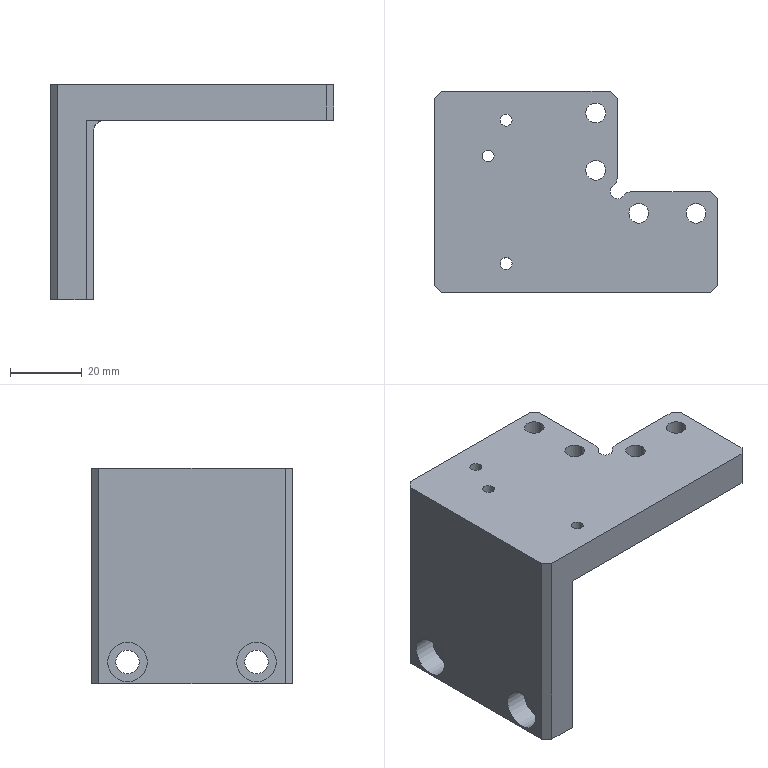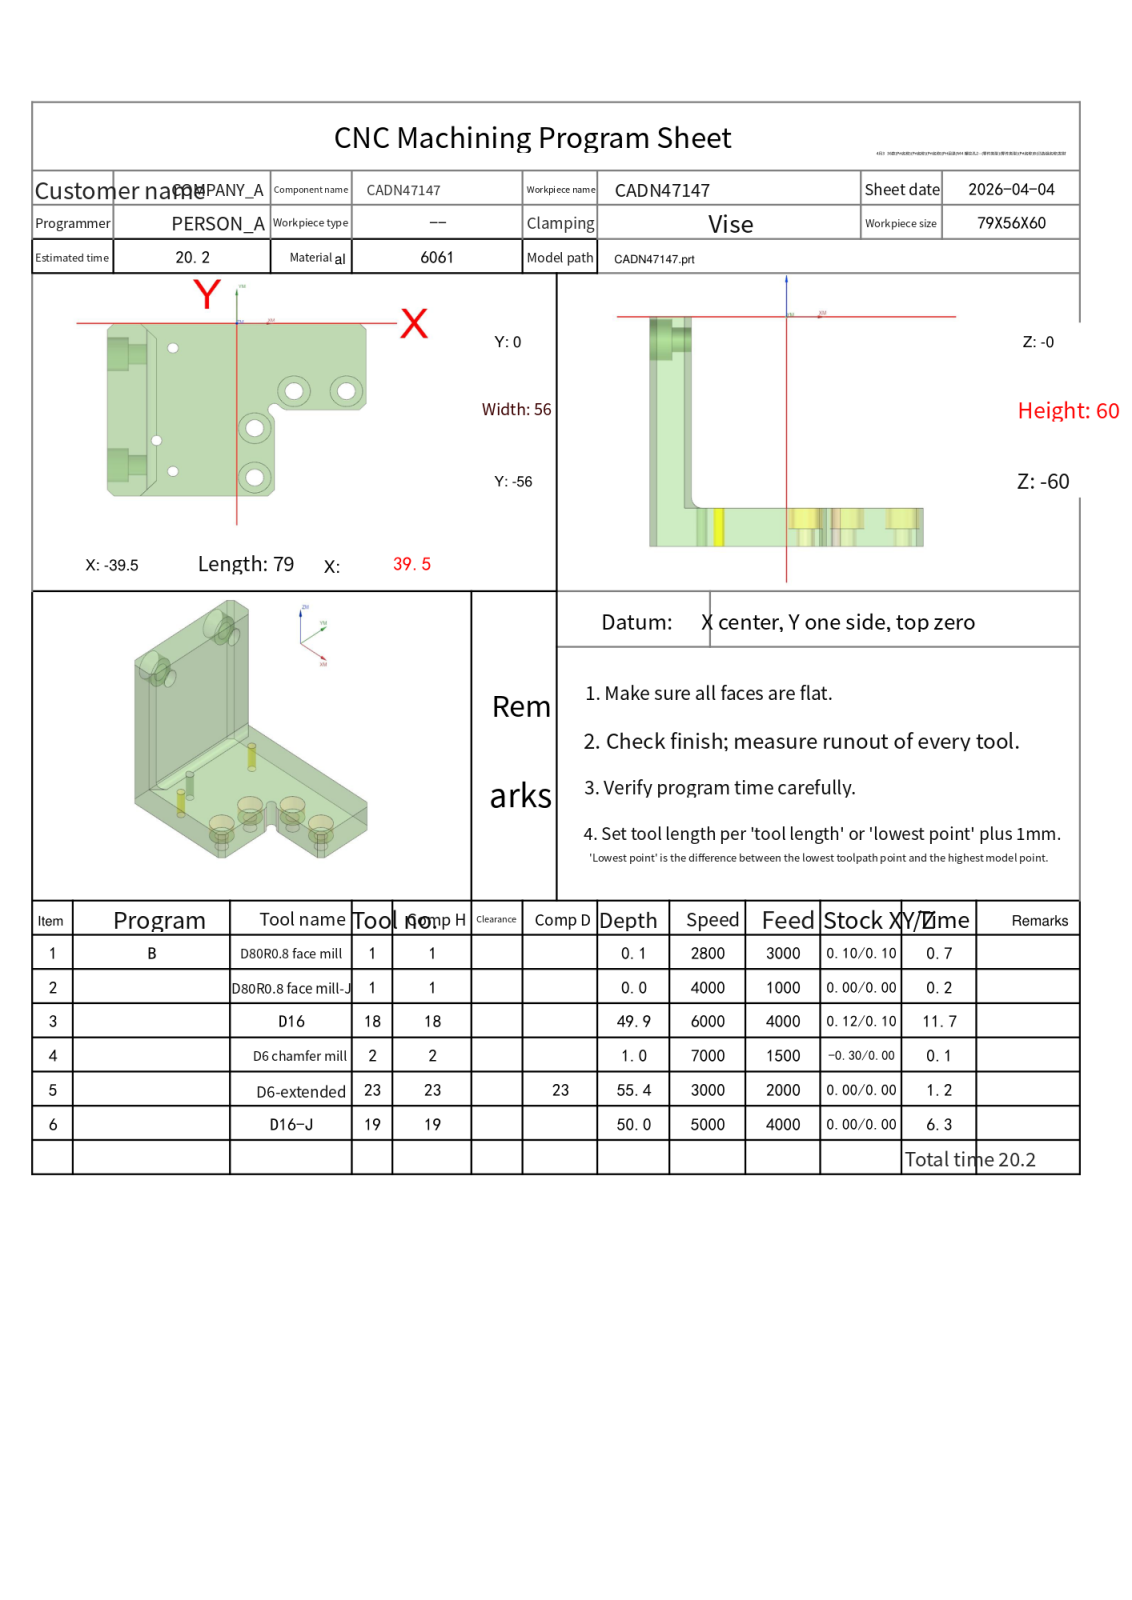NC program | NX | posted by the shop | part box 79 x 56 x 60 mm
Lines 11359 to 12639 of 15895:
N6 T19 M06
(D16-J  D=16. R=0. H=19 ce=0.40 di=0.00)
G00 G90 G54 X-.77 Y11.2 M03 S5000
G43 H19 Z14.5
M08
Z-48.5
G01 Z-50. F1000.
Y4.8
G03 X2.43 Y1.6 I3.2 J0.0
G01 X37.503
G02 X38.629 Y1.134 I-.003 J-1.6
G01 X40.634 Y-.871
G02 X41.1 Y-1.997 I-1.134 J-1.129
G01 Y-26.003
G02 X40.634 Y-27.129 I-1.6 J.003
G01 X38.629 Y-29.134
G02 X37.503 Y-29.6 I-1.129 J1.134
G01 X13.1
Y-54.003
G02 X12.634 Y-55.129 I-1.6 J.003
G01 X10.629 Y-57.134
G02 X9.503 Y-57.6 I-1.129 J1.134
G01 X-18.45
G02 X-18.768 Y-57.28 I.001 J.32
X-18.675 Y-57.055 I.32 J0.0
G01 X-16.1 Y-54.479
Y-1.521
X-18.675 Y1.055
G02 X-18.768 Y1.28 I.227 J.225
X-18.45 Y1.6 I.32 J0.0
G01 X5.768
G02 X6.898 Y1.132 I-.001 J-1.6
G01 X13.962 Y-5.932
G03 X15.092 Y-6.4 I1.131 J1.132
G01 X31.504
G02 X33.1 Y-7.996 I-.004 J-1.6
G01 Y-20.004
G02 X31.504 Y-21.6 I-1.6 J.004
G01 X13.1
G03 X5.1 Y-29.6 I0.0 J-8.
G01 Y-48.004
G02 X3.504 Y-49.6 I-1.6 J.004
G01 X-6.504
G02 X-8.1 Y-48.004 I.004 J1.6
G01 Y-7.996
G02 X-6.504 Y-6.4 I1.6 J-.004
G01 X4.94
G02 X6.06 Y-7.52 I0.0 J-1.12
X6.016 Y-7.831 I-1.12 J0.0
G01 X4.266 Y-13.878
G03 X4.203 Y-14.322 I1.537 J-.444
X4.367 Y-15.027 I1.6 J0.0
G02 X4.481 Y-15.52 I-1.005 J-.493
X4.001 Y-16.439 I-1.12 J0.0
G03 X2.552 Y-17.569 I9.099 J-13.161
G02 X1.5 Y-17.964 I-1.052 J1.206
X-.1 Y-16.367 I0.0 J1.6
G01 Y-15.996
G02 X1.496 Y-14.4 I1.6 J-.004
G01 X3.364
G02 X4.047 Y-14.635 I-.003 J-1.12
X4.481 Y-15.499 I-.686 J-.885
G03 X7.68 Y-18.64 I3.199 J.059
G01 X7.74 Y-18.639
Z-48.5
G00 Z14.5
G00 G90 X-23.903 Y9.001 M03 S5000
Z9.5
Z-8.4
G01 Z-9.4 F1000.
G41 D19
X-24.028 Y8.844
G03 X-24.546 Y7.354 I1.882 J-1.49
X-23.843 Y5.657 I2.4 J0.0
G01 X-21.843 Y3.657
G02 X-19.5 Y-2. I-5.657 J-5.657
G01 Y-54.
G02 X-21.847 Y-59.661 I-8. J0.0
G01 X-23.843 Y-61.657
G03 X-24.546 Y-63.354 I1.697 J-1.697
X-24.028 Y-64.844 I2.4 J0.0
G01 G40 X-23.903 Y-65.001
Z-8.4
G00 Z9.5
Y9.001
Z-17.8
G01 Z-18.8
G41 D19
X-24.028 Y8.844
G03 X-24.546 Y7.354 I1.882 J-1.49
X-23.843 Y5.657 I2.4 J0.0
G01 X-21.843 Y3.657
G02 X-19.5 Y-2. I-5.657 J-5.657
G01 Y-54.
G02 X-21.847 Y-59.661 I-8. J0.0
G01 X-23.843 Y-61.657
G03 X-24.546 Y-63.354 I1.697 J-1.697
X-24.028 Y-64.844 I2.4 J0.0
G01 G40 X-23.903 Y-65.001
Z-17.8
G00 Z9.5
Y9.001
Z-27.2
G01 Z-28.2
G41 D19
X-24.028 Y8.844
G03 X-24.546 Y7.354 I1.882 J-1.49
X-23.843 Y5.657 I2.4 J0.0
G01 X-21.843 Y3.657
G02 X-19.5 Y-2. I-5.657 J-5.657
G01 Y-54.
G02 X-21.847 Y-59.661 I-8. J0.0
G01 X-23.843 Y-61.657
G03 X-24.546 Y-63.354 I1.697 J-1.697
X-24.028 Y-64.844 I2.4 J0.0
G01 G40 X-23.903 Y-65.001
Z-27.2
G00 Z9.5
Y9.001
Z-36.6
G01 Z-37.6
G41 D19
X-24.028 Y8.844
G03 X-24.546 Y7.354 I1.882 J-1.49
X-23.843 Y5.657 I2.4 J0.0
G01 X-21.843 Y3.657
G02 X-19.5 Y-2. I-5.657 J-5.657
G01 Y-54.
G02 X-21.847 Y-59.661 I-8. J0.0
G01 X-23.843 Y-61.657
G03 X-24.546 Y-63.354 I1.697 J-1.697
X-24.028 Y-64.844 I2.4 J0.0
G01 G40 X-23.903 Y-65.001
Z-36.6
G00 Z9.5
Y9.001
Z-46.
G01 Z-47.
G41 D19
X-24.028 Y8.844
G03 X-24.546 Y7.354 I1.882 J-1.49
X-23.843 Y5.657 I2.4 J0.0
G01 X-21.843 Y3.657
G02 X-19.5 Y-2. I-5.657 J-5.657
G01 Y-54.
G02 X-21.847 Y-59.661 I-8. J0.0
G01 X-23.843 Y-61.657
G03 X-24.546 Y-63.354 I1.697 J-1.697
X-24.028 Y-64.844 I2.4 J0.0
G01 G40 X-23.903 Y-65.001
Z-46.
G00 Z9.5
G00 G90 X-26.925 Y11.391 M03 S5000
Z14.5
Z-49.
G01 Z-50. F1000.
G41 D19
X-26.983 Y11.2
G03 X-27.124 Y10.263 I3.06 J-.937
X-26.186 Y8. I3.2 J0.0
G01 X-16.5 Y-1.686
Y-54.314
X-26.186 Y-64.
G03 X-27.124 Y-66.263 I2.263 J-2.263
X-26.983 Y-67.2 I3.2 J0.0
G01 G40 X-26.925 Y-67.391
Z-49.
G00 Z14.5
G00 G90 X-34.428 Y16.241 M03 S5000
Z14.5
Z-46.515
G01 Z-47.015 F4000.
X-24.723 Y6.55
X-23.895 Y5.724
X-23.836 Y5.664
X-21.836 Y3.664
X-21.721 Y3.546
G02 X-19.489 Y-2.001 I-5.778 J-5.547
G01 Y-2.032
X-19.49 Y-2.755
Y-53.245
Y-53.642
Y-53.948
Y-54.006
G02 X-21.755 Y-59.582 I-7.994 J0.0
G01 X-21.836 Y-59.664
X-23.836 Y-61.664
X-24.723 Y-62.55
Z-47.03
X-23.836 Y-61.664
X-21.835 Y-59.663
X-21.755 Y-59.582
G03 X-19.49 Y-54.006 I-5.729 J5.576
G01 Y-53.948
Y-53.642
Y-53.248
Y-2.752
X-19.489 Y-2.032
Y-1.999
G03 X-21.721 Y3.546 I-8.006 J0.0
G01 X-21.835 Y3.663
X-23.836 Y5.664
X-23.895 Y5.724
X-24.723 Y6.55
Z-47.045
X-23.895 Y5.724
X-23.836 Y5.664
X-21.835 Y3.663
X-21.721 Y3.546
G02 X-19.489 Y-1.998 I-5.77 J-5.544
G01 Y-2.032
X-19.49 Y-2.488
Y-53.948
X-19.489 Y-54.005
G02 X-21.755 Y-59.582 I-7.996 J0.0
G01 X-21.835 Y-59.663
X-23.836 Y-61.664
X-24.723 Y-62.55
Z-47.06
X-23.836 Y-61.664
X-21.835 Y-59.663
X-21.755 Y-59.582
G03 X-19.489 Y-54.004 I-5.732 J5.578
G01 Y-53.948
Y-2.488
Y-2.042
X-19.488 Y-2.032
Y-2.
G03 X-21.721 Y3.546 I-8.005 J0.0
G01 X-21.835 Y3.663
X-23.836 Y5.664
X-23.895 Y5.724
X-24.723 Y6.55
Z-47.075
X-23.895 Y5.724
X-23.836 Y5.664
X-21.835 Y3.662
X-21.721 Y3.546
G02 X-19.489 Y-1.993 I-5.759 J-5.54
G01 Y-2.072
Y-53.968
Y-54.004
G02 X-21.755 Y-59.582 I-7.998 J0.0
G01 X-21.835 Y-59.662
X-23.836 Y-61.664
X-24.723 Y-62.55
Z-47.09
X-23.836 Y-61.664
X-21.834 Y-59.662
X-21.755 Y-59.582
G03 X-19.489 Y-54.004 I-5.731 J5.578
G01 Y-53.968
Y-2.042
Y-2.006
G03 X-21.721 Y3.546 I-8.023 J0.0
G01 X-21.834 Y3.662
X-23.836 Y5.664
X-23.895 Y5.724
X-24.723 Y6.55
Z-47.105
X-23.895 Y5.724
X-23.836 Y5.664
X-21.834 Y3.662
X-21.721 Y3.546
G02 X-19.488 Y-1.98 I-5.722 J-5.526
G01 Y-2.042
Y-53.968
Y-54.004
G02 X-21.755 Y-59.582 I-7.996 J0.0
G01 X-21.834 Y-59.662
X-23.836 Y-61.664
X-23.895 Y-61.724
X-24.723 Y-62.55
Z-47.12
X-23.895 Y-61.724
X-23.836 Y-61.664
X-21.834 Y-59.661
X-21.755 Y-59.582
G03 X-19.488 Y-54.005 I-5.724 J5.577
G01 Y-53.968
Y-2.042
X-19.487 Y-1.98
G03 X-21.721 Y3.546 I-7.955 J0.0
G01 X-21.834 Y3.661
X-23.836 Y5.664
X-23.895 Y5.724
X-24.723 Y6.55
Z-47.135
X-23.895 Y5.724
X-23.836 Y5.664
X-21.833 Y3.661
X-21.721 Y3.546
G02 X-19.482 Y-2.009 I-5.772 J-5.555
G01 Y-2.031
X-19.487 Y-2.042
Y-53.968
Y-54.006
G02 X-21.755 Y-59.582 I-7.987 J0.0
G01 X-21.833 Y-59.661
X-23.836 Y-61.664
X-23.895 Y-61.724
X-24.723 Y-62.55
Z-47.15
X-23.895 Y-61.724
X-23.836 Y-61.664
X-21.832 Y-59.66
X-21.755 Y-59.582
G03 X-19.486 Y-54.006 I-5.716 J5.575
G01 Y-53.968
Y-2.042
X-19.481 Y-2.031
Y-2.009
G03 X-21.721 Y3.546 I-8.009 J0.0
G01 X-21.832 Y3.66
X-23.836 Y5.664
X-23.895 Y5.724
X-24.723 Y6.55
Z-47.165
X-23.895 Y5.724
X-23.836 Y5.664
X-21.831 Y3.659
X-21.721 Y3.546
G02 X-19.485 Y-1.982 I-5.717 J-5.528
G01 Y-2.042
Y-53.968
Y-54.008
G02 X-21.755 Y-59.582 I-7.978 J0.0
G01 X-21.831 Y-59.659
X-23.836 Y-61.664
X-23.895 Y-61.724
X-24.723 Y-62.55
Z-47.18
X-23.895 Y-61.724
X-23.836 Y-61.664
X-21.83 Y-59.658
X-21.755 Y-59.582
G03 X-19.485 Y-54.009 I-5.703 J5.573
G01 Y-53.968
Y-2.042
X-19.484 Y-1.977
G03 X-21.721 Y3.546 I-7.938 J0.0
G01 X-21.83 Y3.658
X-23.836 Y5.664
X-23.895 Y5.724
X-24.723 Y6.55
Z-47.195
X-23.895 Y5.724
X-23.836 Y5.664
X-21.829 Y3.657
X-21.721 Y3.546
G02 X-19.483 Y-1.973 I-5.689 J-5.519
G01 X-19.484 Y-2.042
Y-53.968
Y-54.01
G02 X-21.755 Y-59.582 I-7.97 J0.0
G01 X-21.829 Y-59.657
X-23.836 Y-61.664
X-23.895 Y-61.724
X-24.723 Y-62.55
Z-47.21
X-23.895 Y-61.724
X-23.836 Y-61.664
X-21.828 Y-59.656
X-21.755 Y-59.582
G03 X-19.483 Y-54.013 I-5.688 J5.569
G01 Y-53.987
Y-2.042
X-19.482 Y-1.971
G03 X-21.721 Y3.546 I-7.919 J0.0
G01 X-21.828 Y3.656
X-23.836 Y5.664
X-23.895 Y5.724
X-24.723 Y6.55
Z-47.225
X-23.895 Y5.724
X-23.836 Y5.664
X-21.827 Y3.655
X-21.721 Y3.546
G02 X-19.576 Y-.779 I-5.686 J-5.514
X-19.482 Y-1.767 I-5.119 J-.989
G01 Y-53.987
Y-54.012
G02 X-21.755 Y-59.582 I-7.959 J0.0
G01 X-21.827 Y-59.655
X-23.836 Y-61.664
X-23.895 Y-61.724
X-24.723 Y-62.55
Z-47.24
X-23.895 Y-61.724
X-23.836 Y-61.664
X-21.826 Y-59.654
X-21.755 Y-59.582
G03 X-19.48 Y-54.013 I-5.679 J5.569
G01 Y-53.987
Y-1.77
G03 X-19.576 Y-.77 I-5.27 J0.0
X-21.721 Y3.546 I-7.829 J-1.199
G01 X-21.826 Y3.654
X-23.836 Y5.664
X-23.895 Y5.724
X-24.723 Y6.55
Z-47.255
X-23.895 Y5.724
X-23.836 Y5.664
X-21.825 Y3.652
X-21.721 Y3.546
G02 X-19.576 Y-.762 I-5.685 J-5.518
X-19.479 Y-1.784 I-5.339 J-1.022
G01 Y-53.987
Y-54.013
G02 X-21.755 Y-59.582 I-7.95 J0.0
G01 X-21.825 Y-59.652
X-23.836 Y-61.664
X-23.895 Y-61.724
X-24.723 Y-62.55
Z-47.27
X-23.895 Y-61.724
X-23.836 Y-61.664
X-21.823 Y-59.651
X-21.755 Y-59.582
G03 X-19.478 Y-54.012 I-5.672 J5.57
G01 Y-53.987
Y-1.789
G03 X-19.576 Y-.753 I-5.508 J0.0
X-21.721 Y3.546 I-7.829 J-1.22
G01 X-21.823 Y3.651
X-23.836 Y5.664
X-23.895 Y5.724
X-24.723 Y6.55
Z-47.285
X-23.895 Y5.724
X-23.836 Y5.664
X-21.821 Y3.649
X-21.721 Y3.546
G02 X-19.47 Y-2.015 I-5.745 J-5.561
G01 Y-2.031
X-19.476 Y-2.051
Y-53.959
X-19.471 Y-53.987
G02 X-21.755 Y-59.582 I-7.997 J.001
G01 X-21.821 Y-59.649
X-23.836 Y-61.664
X-23.895 Y-61.724
X-24.723 Y-62.55
Z-47.299
X-23.895 Y-61.724
X-23.836 Y-61.664
X-21.819 Y-59.647
X-21.755 Y-59.582
G03 X-19.469 Y-53.987 I-5.71 J5.597
G01 X-19.475 Y-53.949
Y-2.051
X-19.469 Y-2.031
Y-2.014
G03 X-21.721 Y3.546 I-7.99 J0.0
G01 X-21.819 Y3.647
X-23.836 Y5.664
X-23.895 Y5.724
X-24.723 Y6.55
Z-47.314
X-23.895 Y5.724
X-23.836 Y5.664
X-21.817 Y3.645
X-21.721 Y3.547
G02 X-19.467 Y-2.014 I-5.735 J-5.561
G01 X-19.468 Y-2.031
X-19.473 Y-2.051
Y-53.949
Y-54.039
G02 X-19.932 Y-56.665 I-7.737 J0.0
X-21.755 Y-59.582 I-7.469 J2.64
G01 X-21.817 Y-59.645
X-23.836 Y-61.664
X-23.895 Y-61.724
X-24.723 Y-62.55
Z-47.329
X-23.895 Y-61.724
X-23.836 Y-61.664
X-21.816 Y-59.644
X-21.755 Y-59.582
G03 X-19.472 Y-54.006 I-5.667 J5.576
G01 Y-53.949
Y-2.051
X-19.466 Y-2.031
Y-2.016
G03 X-21.721 Y3.547 I-7.991 J0.0
G01 X-21.816 Y3.644
X-23.836 Y5.664
X-23.895 Y5.724
X-24.723 Y6.55
Z-47.344
X-23.895 Y5.724
X-23.836 Y5.664
X-21.814 Y3.642
X-21.721 Y3.547
G02 X-19.47 Y-1.994 I-5.694 J-5.54
G01 Y-2.051
Y-53.949
Y-54.004
G02 X-21.755 Y-59.582 I-7.951 J0.0
G01 X-21.814 Y-59.642
X-23.836 Y-61.664
X-23.895 Y-61.724
X-24.723 Y-62.55
Z-47.359
X-23.895 Y-61.724
X-23.836 Y-61.664
X-21.812 Y-59.64
X-21.755 Y-59.582
G03 X-19.576 Y-55.298 I-5.655 J5.572
X-19.465 Y-54.049 I-6.996 J1.25
G01 X-19.466 Y-53.949
X-19.468 Y-53.939
Y-2.051
Y-1.997
G03 X-21.721 Y3.547 I-7.948 J0.0
G01 X-21.812 Y3.64
X-23.836 Y5.664
X-23.895 Y5.724
X-24.723 Y6.55
Z-47.374
X-23.895 Y5.724
X-23.836 Y5.664
X-21.81 Y3.638
X-21.721 Y3.547
G02 X-19.466 Y-2. I-5.698 J-5.547
G01 X-19.467 Y-2.051
Y-53.939
X-19.463 Y-53.987
G02 X-21.755 Y-59.582 I-7.983 J.004
G01 X-21.81 Y-59.638
X-23.836 Y-61.664
X-23.895 Y-61.724
X-24.723 Y-62.55
Z-47.389
X-23.895 Y-61.724
X-23.836 Y-61.664
X-21.809 Y-59.637
X-21.755 Y-59.582
G03 X-19.463 Y-53.987 I-5.681 J5.595
G01 Y-53.959
X-19.465 Y-53.939
Y-2.051
Y-2.002
G03 X-21.721 Y3.547 I-7.952 J0.0
G01 X-21.809 Y3.637
X-23.836 Y5.664
X-23.895 Y5.724
X-24.723 Y6.55
Z-47.404
X-23.895 Y5.724
X-23.836 Y5.664
X-21.807 Y3.635
X-21.721 Y3.547
G02 X-19.463 Y-2.007 I-5.7 J-5.553
G01 Y-2.041
Y-53.967
Y-53.993
G02 X-21.755 Y-59.582 I-7.959 J0.0
G01 X-21.807 Y-59.635
X-23.836 Y-61.664
X-23.895 Y-61.724
X-24.723 Y-62.55
Z-47.419
X-23.895 Y-61.724
X-23.836 Y-61.664
X-21.805 Y-59.633
X-21.755 Y-59.582
G03 X-19.461 Y-53.989 I-5.67 J5.593
G01 Y-53.967
Y-2.061
X-19.46 Y-2.01
G03 X-21.721 Y3.547 I-7.961 J0.0
G01 X-21.805 Y3.633
X-23.836 Y5.664
X-23.895 Y5.724
X-24.723 Y6.55
Z-47.433
X-23.895 Y5.724
X-23.836 Y5.664
X-21.803 Y3.631
X-21.721 Y3.547
G02 X-19.459 Y-2.013 I-5.702 J-5.56
G01 Y-2.033
Y-53.967
Y-53.987
G02 X-21.755 Y-59.582 I-7.964 J0.0
G01 X-21.803 Y-59.631
X-23.836 Y-61.664
X-23.895 Y-61.724
X-24.723 Y-62.55
Z-47.448
X-23.895 Y-61.724
X-23.836 Y-61.664
X-21.802 Y-59.629
X-21.755 Y-59.582
G03 X-19.456 Y-53.982 I-5.672 J5.6
G01 Y-53.966
Y-2.034
Y-2.017
G03 X-21.721 Y3.547 I-7.967 J0.0
G01 X-21.802 Y3.629
X-23.836 Y5.664
X-23.895 Y5.724
X-24.723 Y6.55
Z-47.463
X-23.895 Y5.724
X-23.836 Y5.664
X-21.8 Y3.628
X-21.721 Y3.547
G02 X-19.454 Y-2.019 I-5.701 J-5.566
G01 Y-2.036
Y-53.964
Y-53.978
G02 X-21.755 Y-59.582 I-7.973 J0.0
G01 X-21.8 Y-59.628
X-23.836 Y-61.664
X-23.895 Y-61.724
X-24.723 Y-62.55
Z-47.478
X-23.895 Y-61.724
X-23.836 Y-61.664
X-21.797 Y-59.625
X-21.755 Y-59.582
G03 X-19.452 Y-53.976 I-5.671 J5.606
G01 Y-53.961
Y-2.039
Y-2.022
G03 X-21.721 Y3.547 I-7.968 J0.0
G01 X-21.797 Y3.625
X-23.836 Y5.664
X-23.895 Y5.724
X-24.723 Y6.55
Z-47.493
X-23.895 Y5.724
X-23.836 Y5.664
X-21.794 Y3.622
X-21.721 Y3.547
G02 X-19.449 Y-2.025 I-5.697 J-5.571
G01 Y-2.042
Y-53.958
Y-53.973
G02 X-21.755 Y-59.582 I-7.975 J0.0
G01 X-21.794 Y-59.622
X-23.836 Y-61.664
X-23.895 Y-61.724
X-24.723 Y-62.55
Z-47.507
X-23.895 Y-61.724
X-23.836 Y-61.664
X-21.792 Y-59.619
X-21.755 Y-59.582
G03 X-19.444 Y-53.987 I-5.68 J5.621
G01 X-19.447 Y-53.956
Y-2.044
Y-2.027
G03 X-21.721 Y3.547 I-7.968 J0.0
G01 X-21.792 Y3.619
X-23.836 Y5.664
X-23.895 Y5.724
X-24.723 Y6.55
Z-47.522
X-23.895 Y5.724
X-23.836 Y5.664
X-21.789 Y3.616
X-21.721 Y3.547
G02 X-19.444 Y-2.029 I-5.691 J-5.576
G01 Y-2.047
Y-53.953
X-19.441 Y-53.987
G02 X-21.755 Y-59.582 I-7.987 J.028
G01 X-21.789 Y-59.616
X-23.836 Y-61.664
X-23.895 Y-61.724
X-24.723 Y-62.55
Z-47.537
X-23.895 Y-61.724
X-23.836 Y-61.664
X-21.786 Y-59.614
X-21.755 Y-59.582
G03 X-19.446 Y-54.209 I-5.64 J5.606
G01 X-19.439 Y-53.959
X-19.442 Y-53.949
Y-2.061
Y-2.032
G03 X-21.725 Y3.55 I-7.966 J0.0
G01 X-21.786 Y3.614
X-23.836 Y5.664
X-23.895 Y5.724
X-24.723 Y6.55
Z-47.552
X-23.895 Y5.724
X-23.836 Y5.664
X-21.783 Y3.611
X-21.72 Y3.547
G02 X-19.439 Y-2.034 I-5.684 J-5.581
G01 Y-2.053
Y-53.947
X-19.433 Y-53.969
X-19.444 Y-54.272
G02 X-21.755 Y-59.582 I-7.95 J.302
G01 X-21.783 Y-59.611
X-23.836 Y-61.664
X-23.895 Y-61.724
X-24.723 Y-62.55
Z-47.566
X-23.895 Y-61.724
X-23.836 Y-61.664
X-21.78 Y-59.608
X-21.755 Y-59.582
G03 X-19.442 Y-54.266 I-5.634 J5.613
G01 X-19.43 Y-53.969
X-19.436 Y-53.944
Y-2.056
Y-2.037
G03 X-21.725 Y3.55 I-7.964 J0.0
G01 X-21.78 Y3.608
X-23.836 Y5.664
X-23.895 Y5.724
X-24.723 Y6.55
Z-47.581
X-23.895 Y5.724
X-23.836 Y5.664
X-21.777 Y3.605
X-21.72 Y3.547
G02 X-19.433 Y-2.039 I-5.675 J-5.585
G01 Y-2.071
Y-53.929
Y-53.961
G02 X-21.759 Y-59.585 I-7.963 J0.0
G01 X-21.777 Y-59.605
X-23.836 Y-61.664
X-23.895 Y-61.724
X-24.723 Y-62.55
Z-47.596
X-23.895 Y-61.724
X-23.836 Y-61.664
X-21.83 Y-59.657
X-21.755 Y-59.582
G03 X-19.43 Y-53.96 I-5.636 J5.622
G01 Y-53.938
Y-2.062
Y-2.042
G03 X-21.725 Y3.55 I-7.962 J0.0
G01 X-21.774 Y3.602
X-23.836 Y5.664
X-23.895 Y5.724
X-24.723 Y6.55
Z-47.611
X-23.895 Y5.724
X-23.836 Y5.664
X-21.771 Y3.599
X-21.72 Y3.547
G02 X-19.427 Y-2.044 I-5.668 J-5.591
G01 Y-2.065
Y-53.935
Y-53.958
G02 X-21.771 Y-59.599 I-7.96 J0.0
G01 X-23.836 Y-61.664
X-23.895 Y-61.724
X-24.723 Y-62.55
Z-47.625
X-23.895 Y-61.724
X-23.836 Y-61.664
X-21.755 Y-59.582
G03 X-19.424 Y-53.955 I-5.627 J5.627
G01 Y-53.932
Y-2.068
Y-2.048
G03 X-21.725 Y3.55 I-7.961 J0.0
G01 X-21.768 Y3.596
X-23.836 Y5.664
X-23.895 Y5.724
X-24.723 Y6.55
Z-47.64
X-23.895 Y5.724
X-23.836 Y5.664
X-21.765 Y3.593
X-21.72 Y3.547
G02 X-19.421 Y-2.05 I-5.661 J-5.597
G01 Y-2.071
Y-53.929
X-19.415 Y-53.939
X-19.427 Y-54.248
G02 X-21.765 Y-59.593 I-7.941 J.29
G01 X-23.836 Y-61.664
X-23.895 Y-61.724
X-24.723 Y-62.55
Z-47.655
X-23.895 Y-61.724
X-23.836 Y-61.664
X-21.755 Y-59.582
G03 X-19.416 Y-53.969 I-5.624 J5.637
G01 X-19.414 Y-53.959
X-19.402 Y-53.941
X-19.418 Y-53.926
Y-2.074
Y-2.054
G03 X-21.725 Y3.55 I-7.961 J0.0
G01 X-21.762 Y3.59
X-23.836 Y5.664
X-23.895 Y5.724
X-24.723 Y6.55
Z-47.669
X-23.895 Y5.724
X-23.836 Y5.664
X-21.759 Y3.587
X-21.72 Y3.547
G02 X-19.414 Y-2.057 I-5.656 J-5.604
G01 Y-2.077
Y-53.923
X-19.4 Y-53.928
X-19.408 Y-53.941
X-19.412 Y-53.969
G02 X-21.759 Y-59.587 I-7.965 J.029
G01 X-23.836 Y-61.664
X-23.895 Y-61.724
X-24.723 Y-62.55
Z-47.684
X-23.895 Y-61.724
X-23.836 Y-61.664
X-21.756 Y-59.584
G03 X-19.408 Y-53.969 I-5.629 J5.652
G01 X-19.406 Y-53.94
X-19.411 Y-53.92
Y-2.08
Y-2.061
G03 X-21.72 Y3.547 I-7.963 J0.0
G01 X-21.756 Y3.584
X-23.836 Y5.664
X-23.895 Y5.724
X-24.723 Y6.55
Z-47.698
X-23.895 Y5.724
X-23.836 Y5.664
X-21.754 Y3.581
X-21.72 Y3.547
G02 X-19.412 Y-1.794 I-5.649 J-5.612
G01 X-19.402 Y-2.07
X-19.408 Y-2.082
Y-53.918
X-19.402 Y-53.94
X-19.405 Y-53.959
G02 X-21.754 Y-59.581 I-7.978 J.032
G01 X-23.836 Y-61.664
X-23.895 Y-61.724
X-24.723 Y-62.55
Z-47.713
X-23.895 Y-61.724
X-23.836 Y-61.664
X-21.75 Y-59.577
G03 X-19.402 Y-53.96 I-5.628 J5.652
G01 X-19.398 Y-53.933
X-19.389 Y-53.92
X-19.404 Y-53.914
Y-2.086
X-19.398 Y-2.07
X-19.408 Y-1.789
G03 X-21.72 Y3.547 I-7.961 J-.281
G01 X-21.75 Y3.577
X-23.836 Y5.664
X-23.895 Y5.724
X-24.723 Y6.55
Z-47.727
X-23.895 Y5.724
X-23.836 Y5.664
X-21.746 Y3.573
X-21.72 Y3.547
G02 X-19.398 Y-2.08 I-5.656 J-5.627
G01 X-19.4 Y-2.09
Y-53.9
X-19.385 Y-53.924
X-19.397 Y-53.95
X-19.398 Y-53.96
G02 X-21.746 Y-59.573 I-7.974 J.037
G01 X-23.836 Y-61.664
X-23.895 Y-61.724
X-24.723 Y-62.55
Z-47.742
X-23.895 Y-61.724
X-23.836 Y-61.664
X-21.741 Y-59.569
G03 X-19.395 Y-53.96 I-5.626 J5.649
G01 X-19.392 Y-53.938
X-19.382 Y-53.92
X-19.397 Y-53.905
Y-2.095
X-19.393 Y-2.08
G03 X-21.725 Y3.55 I-7.983 J-.007
G01 X-21.741 Y3.569
X-23.836 Y5.664
X-23.895 Y5.724
X-24.723 Y6.55
Z-47.757
X-23.895 Y5.724
X-23.836 Y5.664
X-21.72 Y3.547
G02 X-19.389 Y-2.08 I-5.657 J-5.64
G01 X-19.393 Y-2.099
Y-53.901
X-19.384 Y-53.94
X-19.391 Y-53.95
G02 X-21.737 Y-59.565 I-7.978 J.036
G01 X-23.836 Y-61.664
X-23.895 Y-61.724
X-24.723 Y-62.55
Z-47.771
X-23.895 Y-61.724
X-23.836 Y-61.664
X-21.733 Y-59.561
G03 X-19.387 Y-53.95 I-5.63 J5.65
G01 X-19.38 Y-53.94
X-19.389 Y-53.897
Y-2.103
X-19.386 Y-2.09
G03 X-21.733 Y3.561 I-7.986 J-.004
G01 X-23.836 Y5.664
X-23.895 Y5.724
X-24.723 Y6.55
Z-47.786
X-23.895 Y5.724
X-23.836 Y5.664
X-21.72 Y3.547
G02 X-19.381 Y-2.06 I-5.652 J-5.649
G01 X-19.385 Y-2.107
Y-53.893
X-19.383 Y-53.906
Y-53.96
G02 X-21.729 Y-59.557 I-7.979 J.054
G01 X-23.836 Y-61.664
X-23.895 Y-61.724
X-24.723 Y-62.55
Z-47.8
X-23.895 Y-61.724
X-23.836 Y-61.664
X-21.725 Y-59.553
G03 X-19.379 Y-53.96 I-5.635 J5.652
G01 X-19.378 Y-53.899
X-19.381 Y-53.889
Y-2.111
X-19.378 Y-2.06
G03 X-21.725 Y3.553 I-7.988 J-.043
G01 X-23.836 Y5.664
X-23.895 Y5.724
X-24.723 Y6.55
Z-47.814
X-23.895 Y5.724
X-23.836 Y5.664
X-21.721 Y3.549
G02 X-19.374 Y-2.06 I-5.645 J-5.657
G01 X-19.37 Y-2.07
X-19.377 Y-2.115
Y-53.885
X-19.373 Y-53.898
X-19.374 Y-53.97
G02 X-21.721 Y-59.549 I-7.986 J.076
G01 X-23.836 Y-61.664
X-23.895 Y-61.724
X-24.723 Y-62.55
Z-47.829
X-23.895 Y-61.724
X-23.836 Y-61.664
X-21.717 Y-59.545
G03 X-19.371 Y-53.96 I-5.641 J5.655
G01 X-19.368 Y-53.902
X-19.373 Y-53.88
Y-2.12
X-19.365 Y-2.07
X-19.371 Y-2.06
G03 X-21.717 Y3.545 I-7.985 J-.049
G01 X-23.836 Y5.664
X-23.895 Y5.724
X-24.723 Y6.55
Z-47.843
X-23.895 Y5.724
X-23.836 Y5.664
X-21.713 Y3.541
G02 X-19.366 Y-2.06 I-5.646 J-5.658
G01 X-19.361 Y-2.07
X-19.369 Y-2.123
Y-53.877
X-19.364 Y-53.905
X-19.367 Y-53.988
G02 X-21.713 Y-59.541 I-7.985 J.102
G01 X-23.836 Y-61.664
X-23.895 Y-61.724
X-24.723 Y-62.55
Z-47.858
X-23.895 Y-61.724
X-23.836 Y-61.664
X-21.696 Y-59.524
G03 X-19.373 Y-54.219 I-5.623 J5.623
G01 X-19.36 Y-53.89
X-19.365 Y-53.873
Y-2.127
X-19.361 Y-2.06
G03 X-21.709 Y3.537 I-7.999 J-.065
G01 X-23.836 Y5.664
X-23.895 Y5.724
X-24.723 Y6.55
Z-47.872
X-23.895 Y5.724
X-23.836 Y5.664
X-21.705 Y3.533
G02 X-19.356 Y-2.12 I-5.656 J-5.664
G01 X-19.36 Y-2.131
Y-53.869
X-19.355 Y-53.9
X-19.37 Y-54.245
G02 X-21.692 Y-59.52 I-7.947 J.35
G01 X-23.836 Y-61.664
X-23.895 Y-61.724
X-24.723 Y-62.55
Z-47.886
X-23.895 Y-61.724
X-23.836 Y-61.664
X-21.688 Y-59.516
G03 X-19.364 Y-54.201 I-5.626 J5.626
G01 X-19.351 Y-53.88
X-19.356 Y-53.865
Y-2.135
X-19.351 Y-2.12
G03 X-21.701 Y3.529 I-8.009 J-.019
G01 X-23.836 Y5.664
X-23.895 Y5.724
X-24.723 Y6.55
Z-47.901
X-23.895 Y5.724
X-23.836 Y5.664
X-21.697 Y3.525
G02 X-19.348 Y-2.13 I-5.652 J-5.663
G01 X-19.352 Y-2.139
Y-53.861
X-19.347 Y-53.88
X-19.359 Y-54.191
G02 X-21.685 Y-59.513 I-7.957 J.309
G01 X-23.836 Y-61.664
X-23.895 Y-61.724
X-24.723 Y-62.55
Z-47.915
X-23.895 Y-61.724
X-23.836 Y-61.664
X-21.693 Y-59.521
G03 X-19.344 Y-53.97 I-5.653 J5.665
G01 X-19.343 Y-53.87
X-19.347 Y-53.857
Y-2.143
X-19.343 Y-2.13
G03 X-21.693 Y3.521 I-8.003 J-.014
G01 X-23.836 Y5.664
X-23.895 Y5.724
X-24.723 Y6.55
Z-47.929
X-23.895 Y5.724
X-23.836 Y5.664
X-21.688 Y3.516
G02 X-19.338 Y-2.13 I-5.659 J-5.668
G01 X-19.342 Y-2.148
Y-53.852
X-19.338 Y-53.87
X-19.339 Y-53.97
G02 X-21.688 Y-59.516 I-8.007 J.122
G01 X-23.836 Y-61.664
X-23.895 Y-61.724
X-24.723 Y-62.55
Z-47.943
X-23.895 Y-61.724
X-23.836 Y-61.664
X-21.683 Y-59.511
G03 X-19.417 Y-54.979 I-5.622 J5.644
X-19.333 Y-53.899 I-6.936 J1.08
G01 Y-53.87
X-19.338 Y-53.847
Y-2.153
X-19.333 Y-2.129
G03 X-21.683 Y3.511 I-8.009 J-.027
G01 X-23.836 Y5.664
X-23.895 Y5.724
X-24.723 Y6.55
Z-47.958
X-23.895 Y5.724
X-23.836 Y5.664
X-21.678 Y3.506
G02 X-19.329 Y-2.129 I-5.662 J-5.668
G01 X-19.333 Y-2.158
Y-53.842
X-19.331 Y-53.855
Y-53.959
G02 X-19.413 Y-54.979 I-6.372 J0.0
X-21.678 Y-59.506 I-7.889 J1.117
G01 X-23.836 Y-61.664
X-23.895 Y-61.724
X-24.723 Y-62.55
Z-47.972
X-23.895 Y-61.724
X-23.836 Y-61.664
X-21.673 Y-59.501
G03 X-19.408 Y-54.979 I-5.634 J5.65
X-19.326 Y-53.954 I-6.343 J1.025
G01 Y-53.855
X-19.328 Y-53.837
Y-2.163
X-19.323 Y-2.119
G03 X-21.673 Y3.501 I-8.019 J-.052
G01 X-23.836 Y5.664
X-23.895 Y5.724
X-24.723 Y6.55
Z-47.986
X-23.895 Y5.724
X-23.836 Y5.664
X-21.667 Y3.495
G02 X-19.318 Y-2.119 I-5.666 J-5.67
G01 X-19.323 Y-2.168
Y-53.832
X-19.321 Y-53.855
X-19.32 Y-53.949
G02 X-19.403 Y-54.979 I-6.479 J0.0
X-21.667 Y-59.495 I-7.907 J1.139
G01 X-23.836 Y-61.664
X-23.895 Y-61.724
X-24.723 Y-62.55
Z-48.
X-23.895 Y-61.724
X-23.836 Y-61.664
X-21.662 Y-59.49
G03 X-19.398 Y-54.979 I-5.649 J5.659
X-19.316 Y-53.855 I-7.827 J1.136
G01 X-19.318 Y-53.826
Y-2.174
X-19.313 Y-2.119
G03 X-21.662 Y3.49 I-8.013 J-.059
G01 X-23.836 Y5.664
X-23.895 Y5.724
X-24.723 Y6.55
Z-48.014
X-23.895 Y5.724
X-23.836 Y5.664
X-21.657 Y3.485
G02 X-19.309 Y-2.119 I-5.659 J-5.665
G01 X-19.313 Y-2.179
Y-53.821
X-19.311 Y-53.855
G02 X-19.393 Y-54.979 I-7.815 J.006
X-21.657 Y-59.485 I-7.919 J1.157
G01 X-23.836 Y-61.664
X-23.895 Y-61.724
X-24.723 Y-62.55
Z-48.028
X-23.895 Y-61.724
X-23.836 Y-61.664
X-21.652 Y-59.48
G03 X-19.388 Y-54.979 I-5.66 J5.667
X-19.306 Y-53.855 I-7.645 J1.125
G01 X-19.308 Y-53.816
Y-2.184
X-19.304 Y-2.109
G03 X-21.652 Y3.48 I-8.002 J-.074
G01 X-23.836 Y5.664
X-23.895 Y5.724
X-24.723 Y6.55
Z-48.042
X-23.895 Y5.724
X-23.836 Y5.664
X-21.647 Y3.475
G02 X-19.299 Y-2.119 I-5.65 J-5.66
G01 X-19.303 Y-2.189
Y-53.811
X-19.3 Y-53.931
X-19.318 Y-54.417
G02 X-21.647 Y-59.475 I-8.006 J.621
G01 X-23.836 Y-61.664
X-23.895 Y-61.724
X-24.723 Y-62.55
Z-48.056
X-23.895 Y-61.724
X-23.836 Y-61.664
X-21.632 Y-59.46
G03 X-19.536 Y-55.748 I-5.624 J5.624
G01 X-19.484 Y-55.541
G03 X-19.297 Y-53.917 I-6.944 J1.624
G01 X-19.298 Y-53.806
Y-2.194
X-19.294 Y-2.129
G03 X-21.641 Y3.469 I-7.992 J-.059
G01 X-23.836 Y5.664
X-23.895 Y5.724
X-24.723 Y6.55
Z-48.07
X-23.895 Y5.724
X-23.836 Y5.664
X-21.636 Y3.464
G02 X-19.289 Y-2.069 I-5.656 J-5.664
G01 X-19.293 Y-2.199
Y-53.897
G02 X-19.697 Y-56.315 I-7.426 J0.0
G01 X-19.739 Y-56.437
G02 X-21.623 Y-59.451 I-7.471 J2.574
G01 X-23.836 Y-61.664
X-23.895 Y-61.724
X-24.723 Y-62.55
Z-48.084
X-23.895 Y-61.724
X-23.836 Y-61.664
X-21.631 Y-59.459
G03 X-20.352 Y-57.789 I-5.582 J5.602
X-19.287 Y-53.847 I-6.766 J3.943
G01 Y-53.795
Y-2.205
X-19.285 Y-2.129
G03 X-21.631 Y3.459 I-7.984 J-.066
G01 X-23.836 Y5.664
X-23.895 Y5.724
X-24.723 Y6.55
Z-48.098
X-23.895 Y5.724
X-23.836 Y5.664
X-21.626 Y3.454
G02 X-19.282 Y-2.18 I-5.597 J-5.634
G01 Y-2.21
Y-53.79
Y-53.826
G02 X-21.266 Y-59.068 I-7.917 J0.0
G01 X-21.626 Y-59.454
X-23.836 Y-61.664
X-23.895 Y-61.724
X-24.723 Y-62.55
Z-48.112
X-23.895 Y-61.724
X-23.836 Y-61.664
X-21.621 Y-59.449
G03 X-19.276 Y-53.81 I-5.607 J5.638
G01 Y-53.785
Y-2.215
Y-2.19
G03 X-21.621 Y3.449 I-7.951 J0.0
G01 X-23.836 Y5.664
X-23.895 Y5.724
X-24.723 Y6.55
Z-48.126
X-23.895 Y5.724
X-23.836 Y5.664
X-21.616 Y3.444
G02 X-19.271 Y-2.194 I-5.603 J-5.637
G01 Y-2.22
Y-53.78
Y-53.803
G02 X-21.616 Y-59.444 I-7.955 J0.0
G01 X-23.836 Y-61.664
X-23.895 Y-61.724
X-24.723 Y-62.55
Z-48.14
X-23.895 Y-61.724
X-23.836 Y-61.664
X-21.611 Y-59.438
G03 X-19.265 Y-53.798 I-5.609 J5.641
G01 Y-53.775
Y-2.225
Y-2.201
G03 X-21.611 Y3.438 I-7.952 J0.0
G01 X-23.836 Y5.664
X-23.895 Y5.724
X-24.723 Y6.55
Z-48.154
X-23.895 Y5.724
X-23.836 Y5.664
X-21.605 Y3.433
G02 X-19.259 Y-2.211 I-5.617 J-5.644
G01 Y-2.231
Y-53.769
Y-53.788
G02 X-21.605 Y-59.433 I-7.965 J0.0
G01 X-23.836 Y-61.664
X-23.895 Y-61.724
X-24.723 Y-62.55
Z-48.168
X-23.895 Y-61.724
X-23.836 Y-61.664
X-21.599 Y-59.426
G03 X-19.253 Y-53.781 I-5.622 J5.645
G01 Y-53.763
Y-2.237